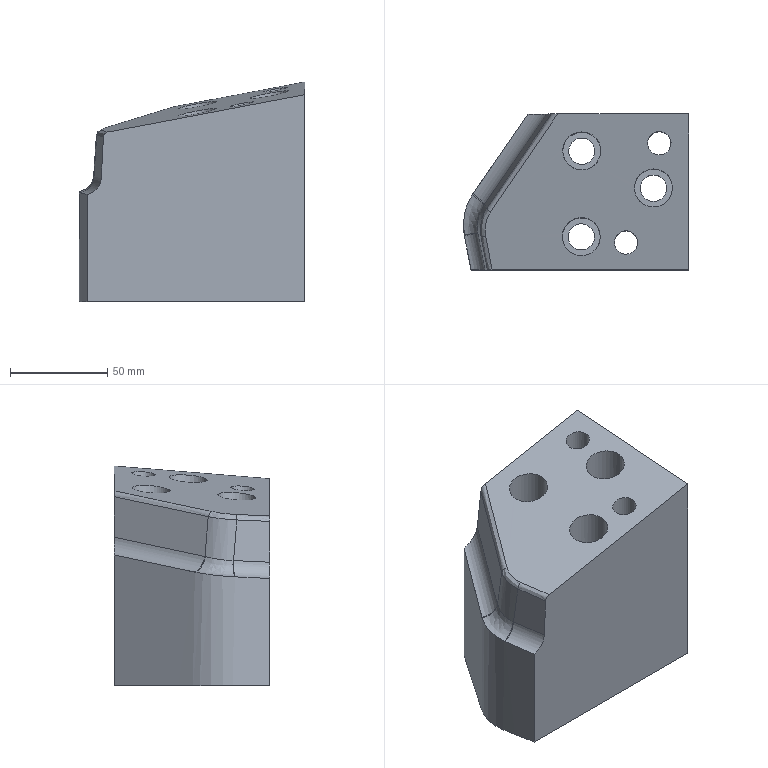Part | NX | features solid 2 | 1 solid | 31 faces | box 115.605 x 80 x 112.905 mm | volume 705851 mm3 | plane 12 | cylinder 11 | spline 8 | commonest cylinder face diameters 13.5 x3 19.5 x3 12 x2 18 x2 40 x1
STEP:
#1=CARTESIAN_POINT('',(809.023,6.563,18.479));
#2=VERTEX_POINT('',#1);
#3=CARTESIAN_POINT('',(809.318,7.001,18.57));
#4=VERTEX_POINT('',#3);
#5=CARTESIAN_POINT('',(833.818,-9.399,21.884));
#6=DIRECTION('',(-0.1858,-0.0797,0.9794));
#7=DIRECTION('',(0.9826,-0.01961,0.1848));
#8=AXIS2_PLACEMENT_3D('',#5,#6,#7);
#9=ELLIPSE('',#8,29.954,29.);
#10=EDGE_CURVE('',#2,#4,#9,.F.);
#11=ORIENTED_EDGE('',*,*,#10,.T.);
#12=CARTESIAN_POINT('',(837.408,48.,27.236));
#13=VERTEX_POINT('',#12);
#14=CARTESIAN_POINT('',(842.075,54.811,28.675));
#15=DIRECTION('',(0.5568,0.8127,0.1718));
#16=VECTOR('',#15,1000.);
#17=LINE('',#14,#16);
#18=EDGE_CURVE('',#4,#13,#17,.T.);
#19=ORIENTED_EDGE('',*,*,#18,.T.);
#20=CARTESIAN_POINT('',(809.023,6.563,18.479));
#21=CARTESIAN_POINT('',(810.152,8.326,18.836));
#22=CARTESIAN_POINT('',(812.578,11.738,19.574));
#23=CARTESIAN_POINT('',(817.289,18.657,21.031));
#24=CARTESIAN_POINT('',(823.217,27.28,22.857));
#25=CARTESIAN_POINT('',(830.31,37.642,25.046));
#26=CARTESIAN_POINT('',(835.042,44.547,26.506));
#27=CARTESIAN_POINT('',(837.408,48.,27.236));
#28=B_SPLINE_CURVE_WITH_KNOTS('',3,(#20,#21,#22,#23,#24,#25,#26,#27),.UNSPECIFIED.,.F.,.F.,(4,1,1,1,1,4),(0.005863,0.01224,0.01861,0.03135,0.0441,0.05684),.UNSPECIFIED.);
#29=EDGE_CURVE('',#2,#13,#28,.T.);
#30=ORIENTED_EDGE('',*,*,#29,.F.);
#31=EDGE_LOOP('',(#11,#19,#30));
#32=FACE_BOUND('',#31,.T.);
#33=CARTESIAN_POINT('',(716.606,144.268,12.152));
#34=DIRECTION('',(-0.1858,-0.0797,0.9794));
#35=DIRECTION('',(-0.9826,0.01961,-0.1848));
#36=AXIS2_PLACEMENT_3D('',#33,#34,#35);
#37=PLANE('',#36);
#38=ADVANCED_FACE('',(#32),#37,.T.);
#39=CARTESIAN_POINT('',(804.902,-14.338,15.996));
#40=VERTEX_POINT('',#39);
#41=CARTESIAN_POINT('',(804.833,-13.968,16.013));
#42=VERTEX_POINT('',#41);
#43=CARTESIAN_POINT('',(804.894,-14.339,15.994));
#44=CARTESIAN_POINT('',(804.873,-14.215,16.001));
#45=CARTESIAN_POINT('',(804.853,-14.092,16.007));
#46=CARTESIAN_POINT('',(804.833,-13.968,16.013));
#47=B_SPLINE_CURVE_WITH_KNOTS('',3,(#43,#44,#45,#46),.UNSPECIFIED.,.F.,.F.,(4,4),(-0.01586,-0.01549),.UNSPECIFIED.);
#48=EDGE_CURVE('',#40,#42,#47,.T.);
#49=ORIENTED_EDGE('',*,*,#48,.F.);
#50=CARTESIAN_POINT('',(833.818,-9.399,21.884));
#51=DIRECTION('',(-0.1858,-0.0797,0.9794));
#52=DIRECTION('',(0.9826,-0.01961,0.1848));
#53=AXIS2_PLACEMENT_3D('',#50,#51,#52);
#54=ELLIPSE('',#53,29.954,29.);
#55=EDGE_CURVE('',#40,#42,#54,.F.);
#56=ORIENTED_EDGE('',*,*,#55,.T.);
#57=EDGE_LOOP('',(#49,#56));
#58=FACE_BOUND('',#57,.T.);
#59=CARTESIAN_POINT('',(716.606,144.268,12.152));
#60=DIRECTION('',(-0.1858,-0.0797,0.9794));
#61=DIRECTION('',(-0.9826,0.01961,-0.1848));
#62=AXIS2_PLACEMENT_3D('',#59,#60,#61);
#63=PLANE('',#62);
#64=ADVANCED_FACE('',(#58),#63,.T.);
#65=CARTESIAN_POINT('',(808.305,-32.,-40.));
#66=VERTEX_POINT('',#65);
#67=CARTESIAN_POINT('',(808.305,-32.,15.204));
#68=VERTEX_POINT('',#67);
#69=CARTESIAN_POINT('',(808.305,-32.,-20.));
#70=DIRECTION('',(0.,0.,1.));
#71=VECTOR('',#70,1000.);
#72=LINE('',#69,#71);
#73=EDGE_CURVE('',#66,#68,#72,.T.);
#74=ORIENTED_EDGE('',*,*,#73,.T.);
#75=CARTESIAN_POINT('',(808.305,-32.,15.204));
#76=CARTESIAN_POINT('',(807.738,-29.056,15.336));
#77=CARTESIAN_POINT('',(806.883,-24.641,15.533));
#78=CARTESIAN_POINT('',(805.758,-18.752,15.799));
#79=CARTESIAN_POINT('',(805.143,-15.817,15.921));
#80=CARTESIAN_POINT('',(804.894,-14.339,15.994));
#81=B_SPLINE_CURVE_WITH_KNOTS('',3,(#75,#76,#77,#78,#79,#80),.UNSPECIFIED.,.F.,.F.,(4,1,1,4),(-0.03354,-0.0247,-0.02028,-0.01586),.UNSPECIFIED.);
#82=EDGE_CURVE('',#68,#40,#81,.T.);
#83=ORIENTED_EDGE('',*,*,#82,.T.);
#84=ORIENTED_EDGE('',*,*,#48,.T.);
#85=CARTESIAN_POINT('',(804.833,-13.968,16.013));
#86=CARTESIAN_POINT('',(804.264,-10.392,16.196));
#87=CARTESIAN_POINT('',(804.244,-4.977,16.633));
#88=CARTESIAN_POINT('',(806.389,1.977,17.606));
#89=CARTESIAN_POINT('',(808.078,5.085,18.179));
#90=CARTESIAN_POINT('',(809.023,6.563,18.479));
#91=B_SPLINE_CURVE_WITH_KNOTS('',3,(#85,#86,#87,#88,#89,#90),.UNSPECIFIED.,.F.,.F.,(4,1,1,4),(-0.01549,-0.004812,0.0005253,0.005863),.UNSPECIFIED.);
#92=EDGE_CURVE('',#42,#2,#91,.T.);
#93=ORIENTED_EDGE('',*,*,#92,.T.);
#94=ORIENTED_EDGE('',*,*,#29,.T.);
#95=CARTESIAN_POINT('',(837.408,48.,-40.));
#96=VERTEX_POINT('',#95);
#97=CARTESIAN_POINT('',(837.408,48.,-20.));
#98=DIRECTION('',(0.,0.,1.));
#99=VECTOR('',#98,1000.);
#100=LINE('',#97,#99);
#101=EDGE_CURVE('',#96,#13,#100,.T.);
#102=ORIENTED_EDGE('',*,*,#101,.F.);
#103=CARTESIAN_POINT('',(837.408,48.,-40.));
#104=CARTESIAN_POINT('',(835.29,44.909,-40.));
#105=CARTESIAN_POINT('',(831.053,38.726,-40.));
#106=CARTESIAN_POINT('',(824.703,29.448,-40.));
#107=CARTESIAN_POINT('',(818.33,20.188,-40.));
#108=CARTESIAN_POINT('',(813.088,12.42,-40.));
#109=CARTESIAN_POINT('',(808.722,6.332,-40.));
#110=CARTESIAN_POINT('',(805.216,-0.3644,-40.));
#111=CARTESIAN_POINT('',(803.948,-8.039,-40.));
#112=CARTESIAN_POINT('',(805.039,-15.466,-40.));
#113=CARTESIAN_POINT('',(806.576,-22.797,-40.));
#114=CARTESIAN_POINT('',(807.596,-28.322,-40.));
#115=CARTESIAN_POINT('',(808.305,-32.,-40.));
#116=B_SPLINE_CURVE_WITH_KNOTS('',3,(#103,#104,#105,#106,#107,#108,#109,#110,#111,#112,#113,#114,#115),.UNSPECIFIED.,.F.,.F.,(4,1,1,1,1,1,1,1,1,1,4),(0.,0.01124,0.02248,0.03373,0.04497,0.05059,0.05621,0.06745,0.07308,0.0787,0.08994),.UNSPECIFIED.);
#117=EDGE_CURVE('',#96,#66,#116,.T.);
#118=ORIENTED_EDGE('',*,*,#117,.T.);
#119=EDGE_LOOP('',(#74,#83,#84,#93,#94,#102,#118));
#120=FACE_BOUND('',#119,.T.);
#121=CARTESIAN_POINT('',(837.408,48.,-40.));
#122=CARTESIAN_POINT('',(837.408,48.,27.639));
#123=CARTESIAN_POINT('',(833.016,41.59,-40.));
#124=CARTESIAN_POINT('',(833.016,41.59,27.639));
#125=CARTESIAN_POINT('',(823.964,28.378,-40.));
#126=CARTESIAN_POINT('',(823.964,28.378,27.639));
#127=CARTESIAN_POINT('',(814.6,14.711,-40.));
#128=CARTESIAN_POINT('',(814.6,14.711,27.639));
#129=CARTESIAN_POINT('',(808.81,6.296,-40.));
#130=CARTESIAN_POINT('',(808.81,6.296,27.639));
#131=CARTESIAN_POINT('',(807.091,3.369,-40.));
#132=CARTESIAN_POINT('',(807.091,3.369,27.639));
#133=CARTESIAN_POINT('',(805.718,-0.1233,-40.));
#134=CARTESIAN_POINT('',(805.718,-0.1233,27.639));
#135=CARTESIAN_POINT('',(804.681,-4.18,-40.));
#136=CARTESIAN_POINT('',(804.681,-4.18,27.639));
#137=CARTESIAN_POINT('',(804.207,-8.797,-40.));
#138=CARTESIAN_POINT('',(804.207,-8.797,27.639));
#139=CARTESIAN_POINT('',(804.676,-13.4,-40.));
#140=CARTESIAN_POINT('',(804.676,-13.4,27.639));
#141=CARTESIAN_POINT('',(805.747,-18.727,-40.));
#142=CARTESIAN_POINT('',(805.747,-18.727,27.639));
#143=CARTESIAN_POINT('',(806.882,-24.614,-40.));
#144=CARTESIAN_POINT('',(806.882,-24.614,27.639));
#145=CARTESIAN_POINT('',(807.847,-29.624,-40.));
#146=CARTESIAN_POINT('',(807.847,-29.624,27.639));
#147=CARTESIAN_POINT('',(808.305,-32.,-40.));
#148=CARTESIAN_POINT('',(808.305,-32.,27.639));
#149=B_SPLINE_SURFACE_WITH_KNOTS('',3,1,((#121,#122),(#123,#124),(#125,#126),(#127,#128),(#129,#130),(#131,#132),(#133,#134),(#135,#136),(#137,#138),(#139,#140),(#141,#142),(#143,#144),(#145,#146),(#147,#148)),.SURF_OF_LINEAR_EXTRUSION.,.F.,.F.,.F.,(4,1,1,1,1,1,1,1,1,1,1,4),(2,2),(0.4029,0.4529,0.5061,0.5096,0.5187,0.5279,0.5337,0.5457,0.5577,0.5634,0.5807,0.5963),(0.3963,0.7471),.UNSPECIFIED.);
#150=ADVANCED_FACE('',(#120),#149,.T.);
#151=CARTESIAN_POINT('',(819.154,-32.,47.263));
#152=VERTEX_POINT('',#151);
#153=CARTESIAN_POINT('',(920.,-32.,66.395));
#154=VERTEX_POINT('',#153);
#155=CARTESIAN_POINT('',(819.154,-32.,47.263));
#156=CARTESIAN_POINT('',(852.769,-32.,53.64));
#157=CARTESIAN_POINT('',(886.385,-32.,60.017));
#158=CARTESIAN_POINT('',(920.,-32.,66.395));
#159=B_SPLINE_CURVE_WITH_KNOTS('',3,(#155,#156,#157,#158),.UNSPECIFIED.,.F.,.F.,(4,4),(0.,0.1026),.UNSPECIFIED.);
#160=EDGE_CURVE('',#152,#154,#159,.T.);
#161=ORIENTED_EDGE('',*,*,#160,.F.);
#162=CARTESIAN_POINT('',(816.706,-32.,44.488));
#163=VERTEX_POINT('',#162);
#164=CARTESIAN_POINT('',(819.154,-32.,47.263));
#165=CARTESIAN_POINT('',(817.835,-32.,47.012));
#166=CARTESIAN_POINT('',(816.773,-32.,45.829));
#167=CARTESIAN_POINT('',(816.706,-32.,44.488));
#168=B_SPLINE_CURVE_WITH_KNOTS('',3,(#164,#165,#166,#167),.UNSPECIFIED.,.F.,.F.,(4,4),(0.,0.00397),.UNSPECIFIED.);
#169=EDGE_CURVE('',#152,#163,#168,.T.);
#170=ORIENTED_EDGE('',*,*,#169,.T.);
#171=CARTESIAN_POINT('',(815.649,-32.,23.529));
#172=VERTEX_POINT('',#171);
#173=CARTESIAN_POINT('',(812.33,-32.,-42.298));
#174=DIRECTION('',(0.05035,0.,0.9987));
#175=VECTOR('',#174,1000.);
#176=LINE('',#173,#175);
#177=EDGE_CURVE('',#163,#172,#176,.F.);
#178=ORIENTED_EDGE('',*,*,#177,.T.);
#179=CARTESIAN_POINT('',(806.495,-32.,24.051));
#180=DIRECTION('',(0.,-1.,0.));
#181=DIRECTION('',(-0.974,0.,0.2265));
#182=AXIS2_PLACEMENT_3D('',#179,#180,#181);
#183=ELLIPSE('',#182,9.174,9.);
#184=EDGE_CURVE('',#172,#68,#183,.F.);
#185=ORIENTED_EDGE('',*,*,#184,.T.);
#186=ORIENTED_EDGE('',*,*,#73,.F.);
#187=CARTESIAN_POINT('',(920.,-32.,-40.));
#188=VERTEX_POINT('',#187);
#189=CARTESIAN_POINT('',(915.5,-32.,-40.));
#190=DIRECTION('',(-1.,0.,0.));
#191=VECTOR('',#190,1000.);
#192=LINE('',#189,#191);
#193=EDGE_CURVE('',#66,#188,#192,.F.);
#194=ORIENTED_EDGE('',*,*,#193,.T.);
#195=CARTESIAN_POINT('',(920.,-32.,-47.5));
#196=DIRECTION('',(0.,0.,-1.));
#197=VECTOR('',#196,1000.);
#198=LINE('',#195,#197);
#199=EDGE_CURVE('',#154,#188,#198,.T.);
#200=ORIENTED_EDGE('',*,*,#199,.F.);
#201=EDGE_LOOP('',(#161,#170,#178,#185,#186,#194,#200));
#202=FACE_BOUND('',#201,.T.);
#203=CARTESIAN_POINT('',(915.5,-32.,-47.5));
#204=DIRECTION('',(0.,-1.,0.));
#205=DIRECTION('',(-1.,0.,0.));
#206=AXIS2_PLACEMENT_3D('',#203,#204,#205);
#207=PLANE('',#206);
#208=ADVANCED_FACE('',(#202),#207,.T.);
#209=CARTESIAN_POINT('',(818.413,-2.215,49.546));
#210=VERTEX_POINT('',#209);
#211=CARTESIAN_POINT('',(815.825,-14.724,48.037));
#212=VERTEX_POINT('',#211);
#213=CARTESIAN_POINT('',(818.413,-2.215,49.546));
#214=CARTESIAN_POINT('',(815.942,-5.823,48.783));
#215=CARTESIAN_POINT('',(814.985,-10.368,48.232));
#216=CARTESIAN_POINT('',(815.825,-14.724,48.037));
#217=B_SPLINE_CURVE_WITH_KNOTS('',3,(#213,#214,#215,#216),.UNSPECIFIED.,.F.,.F.,(4,4),(0.,0.01313),.UNSPECIFIED.);
#218=EDGE_CURVE('',#210,#212,#217,.T.);
#219=ORIENTED_EDGE('',*,*,#218,.T.);
#220=CARTESIAN_POINT('',(815.825,-14.724,48.037));
#221=CARTESIAN_POINT('',(816.934,-20.483,47.779));
#222=CARTESIAN_POINT('',(818.044,-26.241,47.521));
#223=CARTESIAN_POINT('',(819.154,-32.,47.263));
#224=B_SPLINE_CURVE_WITH_KNOTS('',3,(#220,#221,#222,#223),.UNSPECIFIED.,.F.,.F.,(4,4),(0.,0.01761),.UNSPECIFIED.);
#225=EDGE_CURVE('',#212,#152,#224,.T.);
#226=ORIENTED_EDGE('',*,*,#225,.T.);
#227=ORIENTED_EDGE('',*,*,#160,.T.);
#228=CARTESIAN_POINT('',(920.,48.,72.905));
#229=VERTEX_POINT('',#228);
#230=CARTESIAN_POINT('',(920.,-32.,66.395));
#231=CARTESIAN_POINT('',(920.,-5.333,68.565));
#232=CARTESIAN_POINT('',(920.,21.333,70.735));
#233=CARTESIAN_POINT('',(920.,48.,72.905));
#234=B_SPLINE_CURVE_WITH_KNOTS('',3,(#230,#231,#232,#233),.UNSPECIFIED.,.F.,.F.,(4,4),(0.,0.08026),.UNSPECIFIED.);
#235=EDGE_CURVE('',#154,#229,#234,.T.);
#236=ORIENTED_EDGE('',*,*,#235,.T.);
#237=CARTESIAN_POINT('',(852.818,48.,60.159));
#238=VERTEX_POINT('',#237);
#239=CARTESIAN_POINT('',(852.818,48.,60.159));
#240=CARTESIAN_POINT('',(875.212,48.,64.408));
#241=CARTESIAN_POINT('',(897.606,48.,68.656));
#242=CARTESIAN_POINT('',(920.,48.,72.905));
#243=B_SPLINE_CURVE_WITH_KNOTS('',3,(#239,#240,#241,#242),.UNSPECIFIED.,.F.,.F.,(4,4),(0.0003763,0.06876),.UNSPECIFIED.);
#244=EDGE_CURVE('',#238,#229,#243,.T.);
#245=ORIENTED_EDGE('',*,*,#244,.F.);
#246=CARTESIAN_POINT('',(852.818,48.,60.159));
#247=CARTESIAN_POINT('',(841.35,31.262,56.622));
#248=CARTESIAN_POINT('',(829.882,14.523,53.084));
#249=CARTESIAN_POINT('',(818.413,-2.215,49.546));
#250=B_SPLINE_CURVE_WITH_KNOTS('',3,(#246,#247,#248,#249),.UNSPECIFIED.,.F.,.F.,(4,4),(0.,0.06179),.UNSPECIFIED.);
#251=EDGE_CURVE('',#238,#210,#250,.T.);
#252=ORIENTED_EDGE('',*,*,#251,.T.);
#253=EDGE_LOOP('',(#219,#226,#227,#236,#245,#252));
#254=FACE_BOUND('',#253,.T.);
#255=CARTESIAN_POINT('',(910.176,4.689,67.517));
#256=VERTEX_POINT('',#255);
#257=CARTESIAN_POINT('',(904.312,-0.5268,65.98));
#258=CARTESIAN_POINT('',(911.039,4.097,67.632));
#259=CARTESIAN_POINT('',(912.591,12.271,68.592));
#260=CARTESIAN_POINT('',(907.787,19.138,68.239));
#261=CARTESIAN_POINT('',(899.676,20.525,66.813));
#262=CARTESIAN_POINT('',(892.968,15.903,65.165));
#263=CARTESIAN_POINT('',(891.404,7.747,64.204));
#264=CARTESIAN_POINT('',(896.213,0.8606,64.556));
#265=CARTESIAN_POINT('',(904.312,-0.5268,65.98));
#266=CARTESIAN_POINT('',(911.039,4.097,67.632));
#267=CARTESIAN_POINT('',(912.591,12.271,68.592));
#268=B_SPLINE_CURVE_WITH_KNOTS('',3,(#257,#258,#259,#260,#261,#262,#263,#264,#265,#266,#267),.UNSPECIFIED.,.T.,.F.,(1,1,1,1,1,1,1,1,1,1,1,1,1,1,1),(-0.0231,-0.0154,-0.007701,0.,0.007701,0.0154,0.0231,0.0308,0.03851,0.04621,0.05391,0.06161,0.06931,0.07701,0.08471),.UNSPECIFIED.);
#269=EDGE_CURVE('',#256,#256,#268,.T.);
#270=ORIENTED_EDGE('',*,*,#269,.F.);
#271=EDGE_LOOP('',(#270));
#272=FACE_BOUND('',#271,.T.);
#273=CARTESIAN_POINT('',(874.601,-16.091,59.076));
#274=VERTEX_POINT('',#273);
#275=CARTESIAN_POINT('',(871.629,-23.43,57.915));
#276=CARTESIAN_POINT('',(875.665,-16.236,59.267));
#277=CARTESIAN_POINT('',(873.318,-8.171,59.478));
#278=CARTESIAN_POINT('',(866.002,-4.266,58.407));
#279=CARTESIAN_POINT('',(858.186,-6.577,56.737));
#280=CARTESIAN_POINT('',(854.166,-13.76,55.389));
#281=CARTESIAN_POINT('',(856.494,-21.817,55.175));
#282=CARTESIAN_POINT('',(863.825,-25.735,56.247));
#283=CARTESIAN_POINT('',(871.629,-23.43,57.915));
#284=CARTESIAN_POINT('',(875.665,-16.236,59.267));
#285=CARTESIAN_POINT('',(873.318,-8.171,59.478));
#286=B_SPLINE_CURVE_WITH_KNOTS('',3,(#275,#276,#277,#278,#279,#280,#281,#282,#283,#284,#285),.UNSPECIFIED.,.T.,.F.,(1,1,1,1,1,1,1,1,1,1,1,1,1,1,1),(-0.02311,-0.0154,-0.007702,0.,0.007702,0.0154,0.02311,0.03081,0.03851,0.04621,0.05392,0.06162,0.06932,0.07702,0.08472),.UNSPECIFIED.);
#287=EDGE_CURVE('',#274,#274,#286,.T.);
#288=ORIENTED_EDGE('',*,*,#287,.F.);
#289=EDGE_LOOP('',(#288));
#290=FACE_BOUND('',#289,.T.);
#291=CARTESIAN_POINT('',(874.42,25.901,62.459));
#292=VERTEX_POINT('',#291);
#293=CARTESIAN_POINT('',(870.01,19.371,61.091));
#294=CARTESIAN_POINT('',(875.417,25.536,62.619));
#295=CARTESIAN_POINT('',(874.842,33.891,63.19));
#296=CARTESIAN_POINT('',(868.479,39.284,62.421));
#297=CARTESIAN_POINT('',(860.329,38.624,60.821));
#298=CARTESIAN_POINT('',(854.941,32.466,59.298));
#299=CARTESIAN_POINT('',(855.498,24.125,58.725));
#300=CARTESIAN_POINT('',(861.874,18.715,59.494));
#301=CARTESIAN_POINT('',(870.01,19.371,61.091));
#302=CARTESIAN_POINT('',(875.417,25.536,62.619));
#303=CARTESIAN_POINT('',(874.842,33.891,63.19));
#304=B_SPLINE_CURVE_WITH_KNOTS('',3,(#293,#294,#295,#296,#297,#298,#299,#300,#301,#302,#303),.UNSPECIFIED.,.T.,.F.,(1,1,1,1,1,1,1,1,1,1,1,1,1,1,1),(-0.02311,-0.0154,-0.007702,0.,0.007702,0.0154,0.02311,0.03081,0.03851,0.04621,0.05391,0.06162,0.06932,0.07702,0.08472),.UNSPECIFIED.);
#305=EDGE_CURVE('',#292,#292,#304,.T.);
#306=ORIENTED_EDGE('',*,*,#305,.F.);
#307=EDGE_LOOP('',(#306));
#308=FACE_BOUND('',#307,.T.);
#309=CARTESIAN_POINT('',(900.381,36.794,68.271));
#310=VERTEX_POINT('',#309);
#311=CARTESIAN_POINT('',(904.331,39.565,69.246));
#312=CARTESIAN_POINT('',(899.898,37.213,68.213));
#313=CARTESIAN_POINT('',(898.365,32.347,67.527));
#314=CARTESIAN_POINT('',(900.8,27.795,67.618));
#315=CARTESIAN_POINT('',(905.676,26.363,68.427));
#316=CARTESIAN_POINT('',(910.098,28.715,69.457));
#317=CARTESIAN_POINT('',(911.636,33.57,70.144));
#318=CARTESIAN_POINT('',(909.201,38.133,70.053));
#319=CARTESIAN_POINT('',(904.331,39.565,69.246));
#320=CARTESIAN_POINT('',(899.898,37.213,68.213));
#321=CARTESIAN_POINT('',(898.365,32.347,67.527));
#322=B_SPLINE_CURVE_WITH_KNOTS('',3,(#311,#312,#313,#314,#315,#316,#317,#318,#319,#320,#321),.UNSPECIFIED.,.T.,.F.,(1,1,1,1,1,1,1,1,1,1,1,1,1,1,1),(-0.01422,-0.009478,-0.004739,0.,0.004739,0.009478,0.01422,0.01896,0.02369,0.02843,0.03317,0.03791,0.04265,0.04739,0.05213),.UNSPECIFIED.);
#323=EDGE_CURVE('',#310,#310,#322,.T.);
#324=ORIENTED_EDGE('',*,*,#323,.F.);
#325=EDGE_LOOP('',(#324));
#326=FACE_BOUND('',#325,.T.);
#327=CARTESIAN_POINT('',(882.556,-15.206,60.658));
#328=VERTEX_POINT('',#327);
#329=CARTESIAN_POINT('',(885.863,-11.678,61.572));
#330=CARTESIAN_POINT('',(881.991,-14.889,60.576));
#331=CARTESIAN_POINT('',(881.506,-20.,60.068));
#332=CARTESIAN_POINT('',(884.84,-23.925,60.381));
#333=CARTESIAN_POINT('',(889.875,-24.32,61.305));
#334=CARTESIAN_POINT('',(893.735,-21.111,62.298));
#335=CARTESIAN_POINT('',(894.229,-16.011,62.807));
#336=CARTESIAN_POINT('',(890.89,-12.074,62.494));
#337=CARTESIAN_POINT('',(885.863,-11.678,61.572));
#338=CARTESIAN_POINT('',(881.991,-14.889,60.576));
#339=CARTESIAN_POINT('',(881.506,-20.,60.068));
#340=B_SPLINE_CURVE_WITH_KNOTS('',3,(#329,#330,#331,#332,#333,#334,#335,#336,#337,#338,#339),.UNSPECIFIED.,.T.,.F.,(1,1,1,1,1,1,1,1,1,1,1,1,1,1,1),(-0.01422,-0.009479,-0.004739,0.,0.004739,0.009479,0.01422,0.01896,0.0237,0.02844,0.03318,0.03791,0.04265,0.04739,0.05213),.UNSPECIFIED.);
#341=EDGE_CURVE('',#328,#328,#340,.T.);
#342=ORIENTED_EDGE('',*,*,#341,.F.);
#343=EDGE_LOOP('',(#342));
#344=FACE_BOUND('',#343,.T.);
#345=CARTESIAN_POINT('',(920.361,48.485,73.013));
#346=CARTESIAN_POINT('',(919.989,-34.505,66.189));
#347=CARTESIAN_POINT('',(900.884,48.874,69.349));
#348=CARTESIAN_POINT('',(900.511,-34.116,62.525));
#349=CARTESIAN_POINT('',(894.725,48.997,68.191));
#350=CARTESIAN_POINT('',(894.352,-33.993,61.367));
#351=CARTESIAN_POINT('',(815.079,50.586,53.21));
#352=CARTESIAN_POINT('',(814.706,-32.403,46.386));
#353=B_SPLINE_SURFACE_WITH_KNOTS('',1,1,((#345,#346),(#347,#348),(#349,#350),(#351,#352)),.PLANE_SURF.,.F.,.F.,.F.,(2,1,1,2),(2,2),(-0.109,-0.02619,0.,0.3387),(0.4195,0.7113),.PIECEWISE_BEZIER_KNOTS.);
#354=ADVANCED_FACE('',(#254,#272,#290,#308,#326,#344),#353,.T.);
#355=CARTESIAN_POINT('',(847.08,48.,36.34));
#356=VERTEX_POINT('',#355);
#357=CARTESIAN_POINT('',(849.594,48.,57.125));
#358=VERTEX_POINT('',#357);
#359=CARTESIAN_POINT('',(838.073,48.,-38.136));
#360=DIRECTION('',(-0.1201,0.,-0.9928));
#361=VECTOR('',#360,1000.);
#362=LINE('',#359,#361);
#363=EDGE_CURVE('',#356,#358,#362,.F.);
#364=ORIENTED_EDGE('',*,*,#363,.T.);
#365=CARTESIAN_POINT('',(849.594,48.,57.125));
#366=CARTESIAN_POINT('',(849.689,48.,57.915));
#367=CARTESIAN_POINT('',(850.577,48.,59.325));
#368=CARTESIAN_POINT('',(852.039,48.,60.012));
#369=CARTESIAN_POINT('',(852.818,48.,60.159));
#370=B_SPLINE_CURVE_WITH_KNOTS('',3,(#365,#366,#367,#368,#369),.UNSPECIFIED.,.F.,.F.,(4,1,4),(0.,0.002349,0.004697),.UNSPECIFIED.);
#371=EDGE_CURVE('',#358,#238,#370,.T.);
#372=ORIENTED_EDGE('',*,*,#371,.T.);
#373=ORIENTED_EDGE('',*,*,#244,.T.);
#374=CARTESIAN_POINT('',(920.,48.,-40.));
#375=VERTEX_POINT('',#374);
#376=CARTESIAN_POINT('',(920.,48.,-47.5));
#377=DIRECTION('',(0.,0.,1.));
#378=VECTOR('',#377,1000.);
#379=LINE('',#376,#378);
#380=EDGE_CURVE('',#229,#375,#379,.F.);
#381=ORIENTED_EDGE('',*,*,#380,.T.);
#382=CARTESIAN_POINT('',(915.5,48.,-40.));
#383=DIRECTION('',(1.,0.,0.));
#384=VECTOR('',#383,1000.);
#385=LINE('',#382,#384);
#386=EDGE_CURVE('',#96,#375,#385,.T.);
#387=ORIENTED_EDGE('',*,*,#386,.F.);
#388=ORIENTED_EDGE('',*,*,#101,.T.);
#389=CARTESIAN_POINT('',(836.227,48.,36.202));
#390=DIRECTION('',(0.,1.,0.));
#391=DIRECTION('',(0.9556,0.,0.2948));
#392=AXIS2_PLACEMENT_3D('',#389,#390,#391);
#393=ELLIPSE('',#392,11.074,9.);
#394=EDGE_CURVE('',#13,#356,#393,.F.);
#395=ORIENTED_EDGE('',*,*,#394,.T.);
#396=EDGE_LOOP('',(#364,#372,#373,#381,#387,#388,#395));
#397=FACE_BOUND('',#396,.T.);
#398=CARTESIAN_POINT('',(915.5,48.,-47.5));
#399=DIRECTION('',(0.,1.,0.));
#400=DIRECTION('',(1.,0.,0.));
#401=AXIS2_PLACEMENT_3D('',#398,#399,#400);
#402=PLANE('',#401);
#403=ADVANCED_FACE('',(#397),#402,.T.);
#404=CARTESIAN_POINT('',(871.925,29.,-40.));
#405=VERTEX_POINT('',#404);
#406=CARTESIAN_POINT('',(865.175,29.,-40.));
#407=DIRECTION('',(0.,0.,1.));
#408=DIRECTION('',(1.,0.,0.));
#409=AXIS2_PLACEMENT_3D('',#406,#407,#408);
#410=CIRCLE('',#409,6.75);
#411=EDGE_CURVE('',#405,#405,#410,.F.);
#412=ORIENTED_EDGE('',*,*,#411,.F.);
#413=EDGE_LOOP('',(#412));
#414=FACE_BOUND('',#413,.T.);
#415=CARTESIAN_POINT('',(893.865,-18.,-40.));
#416=VERTEX_POINT('',#415);
#417=CARTESIAN_POINT('',(887.865,-18.,-40.));
#418=DIRECTION('',(0.,0.,1.));
#419=DIRECTION('',(1.,0.,0.));
#420=AXIS2_PLACEMENT_3D('',#417,#418,#419);
#421=CIRCLE('',#420,6.);
#422=EDGE_CURVE('',#416,#416,#421,.T.);
#423=ORIENTED_EDGE('',*,*,#422,.T.);
#424=EDGE_LOOP('',(#423));
#425=FACE_BOUND('',#424,.T.);
#426=CARTESIAN_POINT('',(908.75,10.,-40.));
#427=VERTEX_POINT('',#426);
#428=CARTESIAN_POINT('',(902.,10.,-40.));
#429=DIRECTION('',(0.,0.,1.));
#430=DIRECTION('',(1.,0.,0.));
#431=AXIS2_PLACEMENT_3D('',#428,#429,#430);
#432=CIRCLE('',#431,6.75);
#433=EDGE_CURVE('',#427,#427,#432,.T.);
#434=ORIENTED_EDGE('',*,*,#433,.T.);
#435=EDGE_LOOP('',(#434));
#436=FACE_BOUND('',#435,.T.);
#437=CARTESIAN_POINT('',(911.,32.964,-40.));
#438=VERTEX_POINT('',#437);
#439=CARTESIAN_POINT('',(905.,32.964,-40.));
#440=DIRECTION('',(0.,0.,1.));
#441=DIRECTION('',(1.,0.,0.));
#442=AXIS2_PLACEMENT_3D('',#439,#440,#441);
#443=CIRCLE('',#442,6.);
#444=EDGE_CURVE('',#438,#438,#443,.T.);
#445=ORIENTED_EDGE('',*,*,#444,.T.);
#446=EDGE_LOOP('',(#445));
#447=FACE_BOUND('',#446,.T.);
#448=CARTESIAN_POINT('',(871.662,-15.,-40.));
#449=VERTEX_POINT('',#448);
#450=CARTESIAN_POINT('',(864.912,-15.,-40.));
#451=DIRECTION('',(0.,0.,1.));
#452=DIRECTION('',(1.,0.,0.));
#453=AXIS2_PLACEMENT_3D('',#450,#451,#452);
#454=CIRCLE('',#453,6.75);
#455=EDGE_CURVE('',#449,#449,#454,.F.);
#456=ORIENTED_EDGE('',*,*,#455,.F.);
#457=EDGE_LOOP('',(#456));
#458=FACE_BOUND('',#457,.T.);
#459=ORIENTED_EDGE('',*,*,#117,.F.);
#460=ORIENTED_EDGE('',*,*,#386,.T.);
#461=CARTESIAN_POINT('',(920.,8.,-40.));
#462=DIRECTION('',(0.,-1.,0.));
#463=VECTOR('',#462,1000.);
#464=LINE('',#461,#463);
#465=EDGE_CURVE('',#188,#375,#464,.F.);
#466=ORIENTED_EDGE('',*,*,#465,.F.);
#467=ORIENTED_EDGE('',*,*,#193,.F.);
#468=EDGE_LOOP('',(#459,#460,#466,#467));
#469=FACE_BOUND('',#468,.T.);
#470=CARTESIAN_POINT('',(878.5,8.,-40.));
#471=DIRECTION('',(0.,0.,1.));
#472=DIRECTION('',(0.,-1.,0.));
#473=AXIS2_PLACEMENT_3D('',#470,#471,#472);
#474=PLANE('',#473);
#475=ADVANCED_FACE('',(#414,#425,#436,#447,#458,#469),#474,.F.);
#476=ORIENTED_EDGE('',*,*,#465,.T.);
#477=ORIENTED_EDGE('',*,*,#380,.F.);
#478=ORIENTED_EDGE('',*,*,#235,.F.);
#479=ORIENTED_EDGE('',*,*,#199,.T.);
#480=EDGE_LOOP('',(#476,#477,#478,#479));
#481=FACE_BOUND('',#480,.T.);
#482=CARTESIAN_POINT('',(920.,-31.695,100.));
#483=DIRECTION('',(-1.,0.,0.));
#484=DIRECTION('',(0.,0.,1.));
#485=AXIS2_PLACEMENT_3D('',#482,#483,#484);
#486=PLANE('',#485);
#487=ADVANCED_FACE('',(#481),#486,.F.);
#488=CARTESIAN_POINT('',(895.25,10.,-25.));
#489=VERTEX_POINT('',#488);
#490=CARTESIAN_POINT('',(902.,10.,-25.));
#491=DIRECTION('',(0.,0.,-1.));
#492=DIRECTION('',(-1.,0.,0.));
#493=AXIS2_PLACEMENT_3D('',#490,#491,#492);
#494=CIRCLE('',#493,6.75);
#495=EDGE_CURVE('',#489,#489,#494,.F.);
#496=ORIENTED_EDGE('',*,*,#495,.T.);
#497=EDGE_LOOP('',(#496));
#498=FACE_BOUND('',#497,.T.);
#499=ORIENTED_EDGE('',*,*,#433,.F.);
#500=EDGE_LOOP('',(#499));
#501=FACE_BOUND('',#500,.T.);
#502=CARTESIAN_POINT('',(902.,10.,475.649));
#503=DIRECTION('',(0.,0.,-1.));
#504=DIRECTION('',(-1.,0.,0.));
#505=AXIS2_PLACEMENT_3D('',#502,#503,#504);
#506=CYLINDRICAL_SURFACE('',#505,6.75);
#507=ADVANCED_FACE('',(#498,#501),#506,.F.);
#508=ORIENTED_EDGE('',*,*,#323,.T.);
#509=EDGE_LOOP('',(#508));
#510=FACE_BOUND('',#509,.T.);
#511=ORIENTED_EDGE('',*,*,#444,.F.);
#512=EDGE_LOOP('',(#511));
#513=FACE_BOUND('',#512,.T.);
#514=CARTESIAN_POINT('',(905.,32.964,460.892));
#515=DIRECTION('',(0.,0.,-1.));
#516=DIRECTION('',(-1.,0.,0.));
#517=AXIS2_PLACEMENT_3D('',#514,#515,#516);
#518=CYLINDRICAL_SURFACE('',#517,6.);
#519=ADVANCED_FACE('',(#510,#513),#518,.F.);
#520=CARTESIAN_POINT('',(858.162,-15.,-25.));
#521=VERTEX_POINT('',#520);
#522=CARTESIAN_POINT('',(864.912,-15.,-25.));
#523=DIRECTION('',(0.,0.,-1.));
#524=DIRECTION('',(-1.,0.,0.));
#525=AXIS2_PLACEMENT_3D('',#522,#523,#524);
#526=CIRCLE('',#525,6.75);
#527=EDGE_CURVE('',#521,#521,#526,.T.);
#528=ORIENTED_EDGE('',*,*,#527,.F.);
#529=EDGE_LOOP('',(#528));
#530=FACE_BOUND('',#529,.T.);
#531=ORIENTED_EDGE('',*,*,#455,.T.);
#532=EDGE_LOOP('',(#531));
#533=FACE_BOUND('',#532,.T.);
#534=CARTESIAN_POINT('',(864.912,-15.,460.932));
#535=DIRECTION('',(0.,0.,-1.));
#536=DIRECTION('',(-1.,0.,0.));
#537=AXIS2_PLACEMENT_3D('',#534,#535,#536);
#538=CYLINDRICAL_SURFACE('',#537,6.75);
#539=ADVANCED_FACE('',(#530,#533),#538,.F.);
#540=ORIENTED_EDGE('',*,*,#341,.T.);
#541=EDGE_LOOP('',(#540));
#542=FACE_BOUND('',#541,.T.);
#543=ORIENTED_EDGE('',*,*,#422,.F.);
#544=EDGE_LOOP('',(#543));
#545=FACE_BOUND('',#544,.T.);
#546=CARTESIAN_POINT('',(887.865,-18.,461.864));
#547=DIRECTION('',(0.,0.,-1.));
#548=DIRECTION('',(-1.,0.,0.));
#549=AXIS2_PLACEMENT_3D('',#546,#547,#548);
#550=CYLINDRICAL_SURFACE('',#549,6.);
#551=ADVANCED_FACE('',(#542,#545),#550,.F.);
#552=CARTESIAN_POINT('',(858.425,29.,-25.));
#553=VERTEX_POINT('',#552);
#554=CARTESIAN_POINT('',(865.175,29.,-25.));
#555=DIRECTION('',(0.,0.,-1.));
#556=DIRECTION('',(-1.,0.,0.));
#557=AXIS2_PLACEMENT_3D('',#554,#555,#556);
#558=CIRCLE('',#557,6.75);
#559=EDGE_CURVE('',#553,#553,#558,.T.);
#560=ORIENTED_EDGE('',*,*,#559,.F.);
#561=EDGE_LOOP('',(#560));
#562=FACE_BOUND('',#561,.T.);
#563=ORIENTED_EDGE('',*,*,#411,.T.);
#564=EDGE_LOOP('',(#563));
#565=FACE_BOUND('',#564,.T.);
#566=CARTESIAN_POINT('',(865.175,29.,458.136));
#567=DIRECTION('',(0.,0.,-1.));
#568=DIRECTION('',(-1.,0.,0.));
#569=AXIS2_PLACEMENT_3D('',#566,#567,#568);
#570=CYLINDRICAL_SURFACE('',#569,6.75);
#571=ADVANCED_FACE('',(#562,#565),#570,.F.);
#572=ORIENTED_EDGE('',*,*,#305,.T.);
#573=EDGE_LOOP('',(#572));
#574=FACE_BOUND('',#573,.T.);
#575=CARTESIAN_POINT('',(855.425,29.,-25.));
#576=VERTEX_POINT('',#575);
#577=CARTESIAN_POINT('',(865.175,29.,-25.));
#578=DIRECTION('',(0.,0.,-1.));
#579=DIRECTION('',(-1.,0.,0.));
#580=AXIS2_PLACEMENT_3D('',#577,#578,#579);
#581=CIRCLE('',#580,9.75);
#582=EDGE_CURVE('',#576,#576,#581,.T.);
#583=ORIENTED_EDGE('',*,*,#582,.T.);
#584=EDGE_LOOP('',(#583));
#585=FACE_BOUND('',#584,.T.);
#586=CARTESIAN_POINT('',(865.175,29.,473.136));
#587=DIRECTION('',(0.,0.,-1.));
#588=DIRECTION('',(-1.,0.,0.));
#589=AXIS2_PLACEMENT_3D('',#586,#587,#588);
#590=CYLINDRICAL_SURFACE('',#589,9.75);
#591=ADVANCED_FACE('',(#574,#585),#590,.F.);
#592=ORIENTED_EDGE('',*,*,#559,.T.);
#593=EDGE_LOOP('',(#592));
#594=FACE_BOUND('',#593,.T.);
#595=ORIENTED_EDGE('',*,*,#582,.F.);
#596=EDGE_LOOP('',(#595));
#597=FACE_BOUND('',#596,.T.);
#598=CARTESIAN_POINT('',(885.,29.,-25.));
#599=DIRECTION('',(0.,0.,-1.));
#600=DIRECTION('',(-1.,0.,0.));
#601=AXIS2_PLACEMENT_3D('',#598,#599,#600);
#602=PLANE('',#601);
#603=ADVANCED_FACE('',(#594,#597),#602,.F.);
#604=ORIENTED_EDGE('',*,*,#287,.T.);
#605=EDGE_LOOP('',(#604));
#606=FACE_BOUND('',#605,.T.);
#607=CARTESIAN_POINT('',(855.162,-15.,-25.));
#608=VERTEX_POINT('',#607);
#609=CARTESIAN_POINT('',(864.912,-15.,-25.));
#610=DIRECTION('',(0.,0.,-1.));
#611=DIRECTION('',(-1.,0.,0.));
#612=AXIS2_PLACEMENT_3D('',#609,#610,#611);
#613=CIRCLE('',#612,9.75);
#614=EDGE_CURVE('',#608,#608,#613,.T.);
#615=ORIENTED_EDGE('',*,*,#614,.T.);
#616=EDGE_LOOP('',(#615));
#617=FACE_BOUND('',#616,.T.);
#618=CARTESIAN_POINT('',(864.912,-15.,475.932));
#619=DIRECTION('',(0.,0.,-1.));
#620=DIRECTION('',(-1.,0.,0.));
#621=AXIS2_PLACEMENT_3D('',#618,#619,#620);
#622=CYLINDRICAL_SURFACE('',#621,9.75);
#623=ADVANCED_FACE('',(#606,#617),#622,.F.);
#624=ORIENTED_EDGE('',*,*,#527,.T.);
#625=EDGE_LOOP('',(#624));
#626=FACE_BOUND('',#625,.T.);
#627=ORIENTED_EDGE('',*,*,#614,.F.);
#628=EDGE_LOOP('',(#627));
#629=FACE_BOUND('',#628,.T.);
#630=CARTESIAN_POINT('',(860.,-15.,-25.));
#631=DIRECTION('',(0.,0.,-1.));
#632=DIRECTION('',(-1.,0.,0.));
#633=AXIS2_PLACEMENT_3D('',#630,#631,#632);
#634=PLANE('',#633);
#635=ADVANCED_FACE('',(#626,#629),#634,.F.);
#636=CARTESIAN_POINT('',(892.25,10.,-25.));
#637=VERTEX_POINT('',#636);
#638=CARTESIAN_POINT('',(902.,10.,-25.));
#639=DIRECTION('',(0.,0.,-1.));
#640=DIRECTION('',(-1.,0.,0.));
#641=AXIS2_PLACEMENT_3D('',#638,#639,#640);
#642=CIRCLE('',#641,9.75);
#643=EDGE_CURVE('',#637,#637,#642,.T.);
#644=ORIENTED_EDGE('',*,*,#643,.F.);
#645=EDGE_LOOP('',(#644));
#646=FACE_BOUND('',#645,.T.);
#647=ORIENTED_EDGE('',*,*,#495,.F.);
#648=EDGE_LOOP('',(#647));
#649=FACE_BOUND('',#648,.T.);
#650=CARTESIAN_POINT('',(902.,-0.9737,-25.));
#651=DIRECTION('',(0.,0.,-1.));
#652=DIRECTION('',(-1.,0.,0.));
#653=AXIS2_PLACEMENT_3D('',#650,#651,#652);
#654=PLANE('',#653);
#655=ADVANCED_FACE('',(#646,#649),#654,.F.);
#656=ORIENTED_EDGE('',*,*,#269,.T.);
#657=EDGE_LOOP('',(#656));
#658=FACE_BOUND('',#657,.T.);
#659=ORIENTED_EDGE('',*,*,#643,.T.);
#660=EDGE_LOOP('',(#659));
#661=FACE_BOUND('',#660,.T.);
#662=CARTESIAN_POINT('',(902.,10.,475.649));
#663=DIRECTION('',(0.,0.,-1.));
#664=DIRECTION('',(-1.,0.,0.));
#665=AXIS2_PLACEMENT_3D('',#662,#663,#664);
#666=CYLINDRICAL_SURFACE('',#665,9.75);
#667=ADVANCED_FACE('',(#658,#661),#666,.F.);
#668=ORIENTED_EDGE('',*,*,#82,.F.);
#669=CARTESIAN_POINT('',(772.367,154.502,23.563));
#670=DIRECTION('',(-0.189,0.981,0.04397));
#671=VECTOR('',#670,1000.);
#672=LINE('',#669,#671);
#673=EDGE_CURVE('',#68,#40,#672,.T.);
#674=ORIENTED_EDGE('',*,*,#673,.T.);
#675=EDGE_LOOP('',(#668,#674));
#676=FACE_BOUND('',#675,.T.);
#677=CARTESIAN_POINT('',(716.606,144.268,12.152));
#678=DIRECTION('',(-0.1858,-0.0797,0.9794));
#679=DIRECTION('',(-0.9826,0.01961,-0.1848));
#680=AXIS2_PLACEMENT_3D('',#677,#678,#679);
#681=PLANE('',#680);
#682=ADVANCED_FACE('',(#676),#681,.T.);
#683=CARTESIAN_POINT('',(816.479,-0.3324,46.909));
#684=VERTEX_POINT('',#683);
#685=CARTESIAN_POINT('',(815.121,1.354,26.48));
#686=VERTEX_POINT('',#685);
#687=CARTESIAN_POINT('',(815.392,1.016,30.564));
#688=DIRECTION('',(-0.06614,0.08207,-0.9944));
#689=VECTOR('',#688,1000.);
#690=LINE('',#687,#689);
#691=EDGE_CURVE('',#684,#686,#690,.T.);
#692=ORIENTED_EDGE('',*,*,#691,.F.);
#693=CARTESIAN_POINT('',(816.479,-0.3324,46.909));
#694=CARTESIAN_POINT('',(827.517,15.778,50.314));
#695=CARTESIAN_POINT('',(838.556,31.889,53.72));
#696=CARTESIAN_POINT('',(849.594,48.,57.125));
#697=B_SPLINE_CURVE_WITH_KNOTS('',3,(#693,#694,#695,#696),.UNSPECIFIED.,.F.,.F.,(4,4),(0.,0.05947),.UNSPECIFIED.);
#698=EDGE_CURVE('',#684,#358,#697,.T.);
#699=ORIENTED_EDGE('',*,*,#698,.T.);
#700=ORIENTED_EDGE('',*,*,#363,.F.);
#701=CARTESIAN_POINT('',(809.38,-7.026,24.709));
#702=DIRECTION('',(0.5568,0.8127,0.1718));
#703=VECTOR('',#702,1000.);
#704=LINE('',#701,#703);
#705=EDGE_CURVE('',#356,#686,#704,.F.);
#706=ORIENTED_EDGE('',*,*,#705,.T.);
#707=EDGE_LOOP('',(#692,#699,#700,#706));
#708=FACE_BOUND('',#707,.T.);
#709=CARTESIAN_POINT('',(809.31,-8.141,30.213));
#710=DIRECTION('',(0.8305,-0.5478,-0.1004));
#711=DIRECTION('',(0.553,0.8326,0.03193));
#712=AXIS2_PLACEMENT_3D('',#709,#710,#711);
#713=PLANE('',#712);
#714=ADVANCED_FACE('',(#708),#713,.F.);
#715=CARTESIAN_POINT('',(812.052,-13.335,24.365));
#716=VERTEX_POINT('',#715);
#717=CARTESIAN_POINT('',(813.441,-15.058,45.247));
#718=VERTEX_POINT('',#717);
#719=CARTESIAN_POINT('',(812.052,-13.335,24.365));
#720=CARTESIAN_POINT('',(812.515,-13.909,31.326));
#721=CARTESIAN_POINT('',(812.978,-14.484,38.287));
#722=CARTESIAN_POINT('',(813.441,-15.058,45.247));
#723=B_SPLINE_CURVE_WITH_KNOTS('',3,(#719,#720,#721,#722),.UNSPECIFIED.,.F.,.F.,(4,4),(-0.000000004,3.393),.UNSPECIFIED.);
#724=EDGE_CURVE('',#716,#718,#723,.T.);
#725=ORIENTED_EDGE('',*,*,#724,.T.);
#726=CARTESIAN_POINT('',(813.441,-15.058,45.247));
#727=CARTESIAN_POINT('',(812.457,-9.939,45.515));
#728=CARTESIAN_POINT('',(813.573,-4.594,46.12));
#729=CARTESIAN_POINT('',(816.479,-0.3324,46.909));
#730=B_SPLINE_CURVE_WITH_KNOTS('',3,(#726,#727,#728,#729),.UNSPECIFIED.,.F.,.F.,(4,4),(0.,0.01563),.UNSPECIFIED.);
#731=EDGE_CURVE('',#718,#684,#730,.T.);
#732=ORIENTED_EDGE('',*,*,#731,.T.);
#733=ORIENTED_EDGE('',*,*,#691,.T.);
#734=CARTESIAN_POINT('',(814.916,1.053,26.394));
#735=VERTEX_POINT('',#734);
#736=CARTESIAN_POINT('',(832.146,-10.117,30.698));
#737=DIRECTION('',(0.2884,0.07718,-0.9544));
#738=DIRECTION('',(0.9575,-0.02791,0.2871));
#739=AXIS2_PLACEMENT_3D('',#736,#737,#738);
#740=ELLIPSE('',#739,21.36,20.);
#741=EDGE_CURVE('',#686,#735,#740,.F.);
#742=ORIENTED_EDGE('',*,*,#741,.T.);
#743=CARTESIAN_POINT('',(812.004,-13.079,24.372));
#744=VERTEX_POINT('',#743);
#745=CARTESIAN_POINT('',(814.916,1.053,26.394));
#746=CARTESIAN_POINT('',(812.201,-3.017,25.245));
#747=CARTESIAN_POINT('',(811.113,-8.133,24.502));
#748=CARTESIAN_POINT('',(812.004,-13.079,24.372));
#749=B_SPLINE_CURVE_WITH_KNOTS('',3,(#745,#746,#747,#748),.UNSPECIFIED.,.F.,.F.,(4,4),(0.,0.01506),.UNSPECIFIED.);
#750=EDGE_CURVE('',#735,#744,#749,.T.);
#751=ORIENTED_EDGE('',*,*,#750,.T.);
#752=CARTESIAN_POINT('',(832.146,-10.117,30.698));
#753=DIRECTION('',(0.2884,0.07718,-0.9544));
#754=DIRECTION('',(0.9575,-0.02791,0.2871));
#755=AXIS2_PLACEMENT_3D('',#752,#753,#754);
#756=ELLIPSE('',#755,21.36,20.);
#757=EDGE_CURVE('',#744,#716,#756,.F.);
#758=ORIENTED_EDGE('',*,*,#757,.T.);
#759=EDGE_LOOP('',(#725,#732,#733,#742,#751,#758));
#760=FACE_BOUND('',#759,.T.);
#761=CARTESIAN_POINT('',(832.334,-10.35,33.528));
#762=DIRECTION('',(0.06614,-0.08207,0.9944));
#763=DIRECTION('',(-0.004476,-0.9966,-0.08195));
#764=AXIS2_PLACEMENT_3D('',#761,#762,#763);
#765=CYLINDRICAL_SURFACE('',#764,20.);
#766=ADVANCED_FACE('',(#760),#765,.T.);
#767=ORIENTED_EDGE('',*,*,#177,.F.);
#768=CARTESIAN_POINT('',(816.706,-32.,44.488));
#769=CARTESIAN_POINT('',(815.617,-26.353,44.741));
#770=CARTESIAN_POINT('',(814.529,-20.705,44.994));
#771=CARTESIAN_POINT('',(813.441,-15.058,45.247));
#772=B_SPLINE_CURVE_WITH_KNOTS('',3,(#768,#769,#770,#771),.UNSPECIFIED.,.F.,.F.,(4,4),(0.,0.01727),.UNSPECIFIED.);
#773=EDGE_CURVE('',#163,#718,#772,.T.);
#774=ORIENTED_EDGE('',*,*,#773,.T.);
#775=ORIENTED_EDGE('',*,*,#724,.F.);
#776=CARTESIAN_POINT('',(816.785,-37.898,23.264));
#777=DIRECTION('',(-0.189,0.981,0.04397));
#778=VECTOR('',#777,1000.);
#779=LINE('',#776,#778);
#780=EDGE_CURVE('',#716,#172,#779,.F.);
#781=ORIENTED_EDGE('',*,*,#780,.T.);
#782=EDGE_LOOP('',(#767,#774,#775,#781));
#783=FACE_BOUND('',#782,.T.);
#784=CARTESIAN_POINT('',(817.012,-38.032,27.234));
#785=DIRECTION('',(0.9803,0.1911,-0.04943));
#786=DIRECTION('',(-0.186,0.9781,0.09309));
#787=AXIS2_PLACEMENT_3D('',#784,#785,#786);
#788=PLANE('',#787);
#789=ADVANCED_FACE('',(#783),#788,.F.);
#790=ORIENTED_EDGE('',*,*,#184,.F.);
#791=ORIENTED_EDGE('',*,*,#780,.F.);
#792=CARTESIAN_POINT('',(812.052,-13.335,24.365));
#793=CARTESIAN_POINT('',(811.939,-13.268,22.386));
#794=CARTESIAN_POINT('',(810.38,-13.394,18.502));
#795=CARTESIAN_POINT('',(806.814,-13.987,16.387));
#796=CARTESIAN_POINT('',(804.902,-14.338,15.996));
#797=B_SPLINE_CURVE_WITH_KNOTS('',3,(#792,#793,#794,#795,#796),.UNSPECIFIED.,.F.,.F.,(4,1,4),(0.,0.5,1.),.UNSPECIFIED.);
#798=EDGE_CURVE('',#40,#716,#797,.F.);
#799=ORIENTED_EDGE('',*,*,#798,.F.);
#800=ORIENTED_EDGE('',*,*,#673,.F.);
#801=EDGE_LOOP('',(#790,#791,#799,#800));
#802=FACE_BOUND('',#801,.T.);
#803=CARTESIAN_POINT('',(770.695,153.785,32.377));
#804=DIRECTION('',(-0.189,0.981,0.04397));
#805=DIRECTION('',(-0.9819,-0.1892,0.));
#806=AXIS2_PLACEMENT_3D('',#803,#804,#805);
#807=CYLINDRICAL_SURFACE('',#806,9.);
#808=ADVANCED_FACE('',(#802),#807,.F.);
#809=ORIENTED_EDGE('',*,*,#798,.T.);
#810=ORIENTED_EDGE('',*,*,#757,.F.);
#811=CARTESIAN_POINT('',(803.161,-14.685,24.827));
#812=DIRECTION('',(0.1761,-0.9833,-0.0466));
#813=DIRECTION('',(0.9843,0.1763,0.));
#814=AXIS2_PLACEMENT_3D('',#811,#812,#813);
#815=CIRCLE('',#814,9.);
#816=EDGE_CURVE('',#42,#744,#815,.T.);
#817=ORIENTED_EDGE('',*,*,#816,.F.);
#818=ORIENTED_EDGE('',*,*,#55,.F.);
#819=EDGE_LOOP('',(#809,#810,#817,#818));
#820=FACE_BOUND('',#819,.T.);
#821=CARTESIAN_POINT('',(812.004,-13.079,24.372));
#822=CARTESIAN_POINT('',(811.598,-12.821,17.39));
#823=CARTESIAN_POINT('',(804.833,-13.968,16.013));
#824=CARTESIAN_POINT('',(812.02,-13.165,24.369));
#825=CARTESIAN_POINT('',(811.616,-12.914,17.386));
#826=CARTESIAN_POINT('',(804.855,-14.091,16.007));
#827=CARTESIAN_POINT('',(812.036,-13.25,24.367));
#828=CARTESIAN_POINT('',(811.635,-13.006,17.382));
#829=CARTESIAN_POINT('',(804.878,-14.214,16.002));
#830=CARTESIAN_POINT('',(812.052,-13.335,24.365));
#831=CARTESIAN_POINT('',(811.654,-13.098,17.378));
#832=CARTESIAN_POINT('',(804.902,-14.338,15.996));
#833=(BOUNDED_SURFACE()B_SPLINE_SURFACE(3,2,((#821,#822,#823),(#824,#825,#826),(#827,#828,#829),(#830,#831,#832)),.UNSPECIFIED.,.F.,.F.,.F.)B_SPLINE_SURFACE_WITH_KNOTS((4,4),(3,3),(3.321,3.334),(0.,1.),.PIECEWISE_BEZIER_KNOTS.)GEOMETRIC_REPRESENTATION_ITEM()RATIONAL_B_SPLINE_SURFACE(((1.,0.7894,1.),(1.,0.7894,1.),(1.,0.7893,1.),(1.,0.7892,1.)))REPRESENTATION_ITEM('')SURFACE());
#834=ADVANCED_FACE('',(#820),#833,.F.);
#835=ORIENTED_EDGE('',*,*,#816,.T.);
#836=ORIENTED_EDGE('',*,*,#750,.F.);
#837=CARTESIAN_POINT('',(807.351,5.845,27.293));
#838=DIRECTION('',(-0.5417,-0.8233,-0.1698));
#839=DIRECTION('',(0.8354,-0.5497,0.));
#840=AXIS2_PLACEMENT_3D('',#837,#838,#839);
#841=CIRCLE('',#840,9.);
#842=EDGE_CURVE('',#2,#735,#841,.T.);
#843=ORIENTED_EDGE('',*,*,#842,.F.);
#844=ORIENTED_EDGE('',*,*,#92,.F.);
#845=EDGE_LOOP('',(#835,#836,#843,#844));
#846=FACE_BOUND('',#845,.T.);
#847=CARTESIAN_POINT('',(804.833,-13.968,16.013));
#848=CARTESIAN_POINT('',(811.598,-12.821,17.39));
#849=CARTESIAN_POINT('',(812.004,-13.079,24.372));
#850=CARTESIAN_POINT('',(804.547,-12.175,16.105));
#851=CARTESIAN_POINT('',(811.34,-11.487,17.478));
#852=CARTESIAN_POINT('',(811.782,-11.845,24.404));
#853=CARTESIAN_POINT('',(804.219,-8.618,16.332));
#854=CARTESIAN_POINT('',(811.094,-8.798,17.624));
#855=CARTESIAN_POINT('',(811.576,-9.384,24.541));
#856=CARTESIAN_POINT('',(804.8,-3.202,16.883));
#857=CARTESIAN_POINT('',(811.569,-4.727,18.044));
#858=CARTESIAN_POINT('',(811.98,-5.654,24.965));
#859=CARTESIAN_POINT('',(806.356,1.898,17.593));
#860=CARTESIAN_POINT('',(812.838,-0.923,18.588));
#861=CARTESIAN_POINT('',(813.066,-2.149,25.576));
#862=CARTESIAN_POINT('',(808.069,5.071,18.176));
#863=CARTESIAN_POINT('',(814.199,1.411,19.06));
#864=CARTESIAN_POINT('',(814.24,0.03934,26.108));
#865=CARTESIAN_POINT('',(809.023,6.563,18.479));
#866=CARTESIAN_POINT('',(814.975,2.482,19.276));
#867=CARTESIAN_POINT('',(814.916,1.053,26.394));
#868=(BOUNDED_SURFACE()B_SPLINE_SURFACE(3,2,((#847,#848,#849),(#850,#851,#852),(#853,#854,#855),(#856,#857,#858),(#859,#860,#861),(#862,#863,#864),(#865,#866,#867)),.UNSPECIFIED.,.F.,.F.,.F.)B_SPLINE_SURFACE_WITH_KNOTS((4,1,1,1,4),(3,3),(0.0165,0.0219,0.02729,0.03269,0.03809),(0.,1.),.UNSPECIFIED.)GEOMETRIC_REPRESENTATION_ITEM()RATIONAL_B_SPLINE_SURFACE(((1.,0.7894,1.),(1.,0.7915,1.),(1.,0.7912,1.),(1.,0.7897,1.),(1.,0.7853,1.),(1.,0.7817,1.),(1.,0.7783,1.)))REPRESENTATION_ITEM('')SURFACE());
#869=ADVANCED_FACE('',(#846),#868,.F.);
#870=ORIENTED_EDGE('',*,*,#842,.T.);
#871=ORIENTED_EDGE('',*,*,#741,.F.);
#872=CARTESIAN_POINT('',(807.646,6.284,27.384));
#873=DIRECTION('',(-0.5568,-0.8127,-0.1718));
#874=DIRECTION('',(0.8249,-0.5652,0.));
#875=AXIS2_PLACEMENT_3D('',#872,#873,#874);
#876=CIRCLE('',#875,9.);
#877=EDGE_CURVE('',#4,#686,#876,.T.);
#878=ORIENTED_EDGE('',*,*,#877,.F.);
#879=ORIENTED_EDGE('',*,*,#10,.F.);
#880=EDGE_LOOP('',(#870,#871,#878,#879));
#881=FACE_BOUND('',#880,.T.);
#882=CARTESIAN_POINT('',(815.121,1.354,26.48));
#883=CARTESIAN_POINT('',(815.211,2.799,19.346));
#884=CARTESIAN_POINT('',(809.318,7.001,18.57));
#885=CARTESIAN_POINT('',(815.051,1.254,26.451));
#886=CARTESIAN_POINT('',(815.132,2.694,19.323));
#887=CARTESIAN_POINT('',(809.218,6.856,18.54));
#888=CARTESIAN_POINT('',(814.983,1.154,26.423));
#889=CARTESIAN_POINT('',(815.053,2.588,19.299));
#890=CARTESIAN_POINT('',(809.12,6.71,18.509));
#891=CARTESIAN_POINT('',(814.916,1.053,26.394));
#892=CARTESIAN_POINT('',(814.975,2.482,19.276));
#893=CARTESIAN_POINT('',(809.023,6.563,18.479));
#894=(BOUNDED_SURFACE()B_SPLINE_SURFACE(3,2,((#882,#883,#884),(#885,#886,#887),(#888,#889,#890),(#891,#892,#893)),.UNSPECIFIED.,.F.,.F.,.F.)B_SPLINE_SURFACE_WITH_KNOTS((4,4),(3,3),(2.559,2.577),(0.,1.),.PIECEWISE_BEZIER_KNOTS.)GEOMETRIC_REPRESENTATION_ITEM()RATIONAL_B_SPLINE_SURFACE(((1.,0.7775,1.),(1.,0.7778,1.),(1.,0.778,1.),(1.,0.7783,1.)))REPRESENTATION_ITEM('')SURFACE());
#895=ADVANCED_FACE('',(#881),#894,.F.);
#896=ORIENTED_EDGE('',*,*,#877,.T.);
#897=ORIENTED_EDGE('',*,*,#705,.F.);
#898=ORIENTED_EDGE('',*,*,#394,.F.);
#899=ORIENTED_EDGE('',*,*,#18,.F.);
#900=EDGE_LOOP('',(#896,#897,#898,#899));
#901=FACE_BOUND('',#900,.T.);
#902=CARTESIAN_POINT('',(840.403,54.094,37.49));
#903=DIRECTION('',(0.5568,0.8127,0.1718));
#904=DIRECTION('',(-0.8249,0.5652,0.));
#905=AXIS2_PLACEMENT_3D('',#902,#903,#904);
#906=CYLINDRICAL_SURFACE('',#905,9.);
#907=ADVANCED_FACE('',(#901),#906,.F.);
#908=ORIENTED_EDGE('',*,*,#371,.F.);
#909=ORIENTED_EDGE('',*,*,#698,.F.);
#910=CARTESIAN_POINT('',(818.971,-1.976,46.608));
#911=DIRECTION('',(-0.5568,-0.8127,-0.1718));
#912=DIRECTION('',(0.8249,-0.5652,0.));
#913=AXIS2_PLACEMENT_3D('',#910,#911,#912);
#914=CIRCLE('',#913,3.);
#915=EDGE_CURVE('',#210,#684,#914,.T.);
#916=ORIENTED_EDGE('',*,*,#915,.F.);
#917=ORIENTED_EDGE('',*,*,#251,.F.);
#918=EDGE_LOOP('',(#908,#909,#916,#917));
#919=FACE_BOUND('',#918,.T.);
#920=CARTESIAN_POINT('',(818.413,-2.215,49.546));
#921=CARTESIAN_POINT('',(816.449,-0.8143,49.287));
#922=CARTESIAN_POINT('',(816.479,-0.3324,46.909));
#923=CARTESIAN_POINT('',(829.95,14.624,53.105));
#924=CARTESIAN_POINT('',(827.986,16.024,52.846));
#925=CARTESIAN_POINT('',(828.016,16.506,50.468));
#926=CARTESIAN_POINT('',(841.487,31.463,56.664));
#927=CARTESIAN_POINT('',(839.523,32.863,56.405));
#928=CARTESIAN_POINT('',(839.553,33.345,54.027));
#929=CARTESIAN_POINT('',(853.024,48.301,60.223));
#930=CARTESIAN_POINT('',(851.06,49.702,59.964));
#931=CARTESIAN_POINT('',(851.09,50.184,57.586));
#932=(BOUNDED_SURFACE()B_SPLINE_SURFACE(3,2,((#920,#921,#922),(#923,#924,#925),(#926,#927,#928),(#929,#930,#931)),.UNSPECIFIED.,.F.,.F.,.F.)B_SPLINE_SURFACE_WITH_KNOTS((4,4),(3,3),(0.1619,0.224),(0.,1.),.PIECEWISE_BEZIER_KNOTS.)GEOMETRIC_REPRESENTATION_ITEM()RATIONAL_B_SPLINE_SURFACE(((1.,0.7775,1.),(1.,0.7775,1.),(1.,0.7775,1.),(1.,0.7775,1.)))REPRESENTATION_ITEM('')SURFACE());
#933=ADVANCED_FACE('',(#919),#932,.T.);
#934=ORIENTED_EDGE('',*,*,#915,.T.);
#935=ORIENTED_EDGE('',*,*,#731,.F.);
#936=CARTESIAN_POINT('',(813.441,-15.058,45.247));
#937=CARTESIAN_POINT('',(813.516,-15.103,46.567));
#938=CARTESIAN_POINT('',(814.549,-14.958,47.776));
#939=CARTESIAN_POINT('',(815.825,-14.724,48.037));
#940=B_SPLINE_CURVE_WITH_KNOTS('',3,(#936,#937,#938,#939),.UNSPECIFIED.,.F.,.F.,(4,4),(0.,1.),.UNSPECIFIED.);
#941=EDGE_CURVE('',#212,#718,#940,.F.);
#942=ORIENTED_EDGE('',*,*,#941,.F.);
#943=ORIENTED_EDGE('',*,*,#218,.F.);
#944=EDGE_LOOP('',(#934,#935,#942,#943));
#945=FACE_BOUND('',#944,.T.);
#946=CARTESIAN_POINT('',(816.479,-0.3324,46.909));
#947=CARTESIAN_POINT('',(816.449,-0.8143,49.287));
#948=CARTESIAN_POINT('',(818.413,-2.215,49.546));
#949=CARTESIAN_POINT('',(813.578,-4.586,46.122));
#950=CARTESIAN_POINT('',(813.737,-4.93,48.438));
#951=CARTESIAN_POINT('',(815.942,-5.823,48.783));
#952=CARTESIAN_POINT('',(812.456,-9.936,45.515));
#953=CARTESIAN_POINT('',(812.65,-10.184,47.804));
#954=CARTESIAN_POINT('',(814.985,-10.368,48.232));
#955=CARTESIAN_POINT('',(813.441,-15.058,45.247));
#956=CARTESIAN_POINT('',(813.574,-15.137,47.576));
#957=CARTESIAN_POINT('',(815.825,-14.724,48.037));
#958=(BOUNDED_SURFACE()B_SPLINE_SURFACE(3,2,((#946,#947,#948),(#949,#950,#951),(#952,#953,#954),(#955,#956,#957)),.UNSPECIFIED.,.F.,.F.,.F.)B_SPLINE_SURFACE_WITH_KNOTS((4,4),(3,3),(0.,0.01313),(0.,1.),.PIECEWISE_BEZIER_KNOTS.)GEOMETRIC_REPRESENTATION_ITEM()RATIONAL_B_SPLINE_SURFACE(((1.,0.7775,1.),(1.,0.789,1.),(1.,0.7932,1.),(1.,0.7892,1.)))REPRESENTATION_ITEM('')SURFACE());
#959=ADVANCED_FACE('',(#945),#958,.T.);
#960=ORIENTED_EDGE('',*,*,#941,.T.);
#961=ORIENTED_EDGE('',*,*,#773,.F.);
#962=ORIENTED_EDGE('',*,*,#169,.F.);
#963=ORIENTED_EDGE('',*,*,#225,.F.);
#964=EDGE_LOOP('',(#960,#961,#962,#963));
#965=FACE_BOUND('',#964,.T.);
#966=CARTESIAN_POINT('',(819.174,-32.104,47.258));
#967=CARTESIAN_POINT('',(816.923,-32.517,46.797));
#968=CARTESIAN_POINT('',(816.79,-32.438,44.468));
#969=CARTESIAN_POINT('',(818.057,-26.31,47.518));
#970=CARTESIAN_POINT('',(815.806,-26.723,47.057));
#971=CARTESIAN_POINT('',(815.674,-26.645,44.728));
#972=CARTESIAN_POINT('',(816.941,-20.517,47.777));
#973=CARTESIAN_POINT('',(814.69,-20.93,47.317));
#974=CARTESIAN_POINT('',(814.557,-20.851,44.987));
#975=CARTESIAN_POINT('',(815.825,-14.724,48.037));
#976=CARTESIAN_POINT('',(813.574,-15.137,47.576));
#977=CARTESIAN_POINT('',(813.441,-15.058,45.247));
#978=(BOUNDED_SURFACE()B_SPLINE_SURFACE(3,2,((#966,#967,#968),(#969,#970,#971),(#972,#973,#974),(#975,#976,#977)),.UNSPECIFIED.,.F.,.F.,.F.)B_SPLINE_SURFACE_WITH_KNOTS((4,4),(3,3),(0.0639,0.08161),(0.,1.),.PIECEWISE_BEZIER_KNOTS.)GEOMETRIC_REPRESENTATION_ITEM()RATIONAL_B_SPLINE_SURFACE(((1.,0.7892,1.),(1.,0.7892,1.),(1.,0.7892,1.),(1.,0.7892,1.)))REPRESENTATION_ITEM('')SURFACE());
#979=ADVANCED_FACE('',(#965),#978,.T.);
#980=CLOSED_SHELL('',(#38,#64,#150,#208,#354,#403,#475,#487,#507,#519,#539,#551,#571,#591,#603,#623,#635,#655,#667,#682,#714,#766,#789,#808,#834,#869,#895,#907,#933,#959,#979));
#981=MANIFOLD_SOLID_BREP('',#980);
#982=(LENGTH_UNIT()NAMED_UNIT(*)SI_UNIT(.MILLI.,.METRE.));
#983=UNCERTAINTY_MEASURE_WITH_UNIT(LENGTH_MEASURE(0.0508),#982,'','');
#984=(NAMED_UNIT(*)PLANE_ANGLE_UNIT()SI_UNIT($,.RADIAN.));
#985=(NAMED_UNIT(*)SI_UNIT($,.STERADIAN.)SOLID_ANGLE_UNIT());
#986=(GEOMETRIC_REPRESENTATION_CONTEXT(3)GLOBAL_UNCERTAINTY_ASSIGNED_CONTEXT((#983))GLOBAL_UNIT_ASSIGNED_CONTEXT((#982,#984,#985))REPRESENTATION_CONTEXT('',''));
#987=ADVANCED_BREP_SHAPE_REPRESENTATION('',(#981),#986);